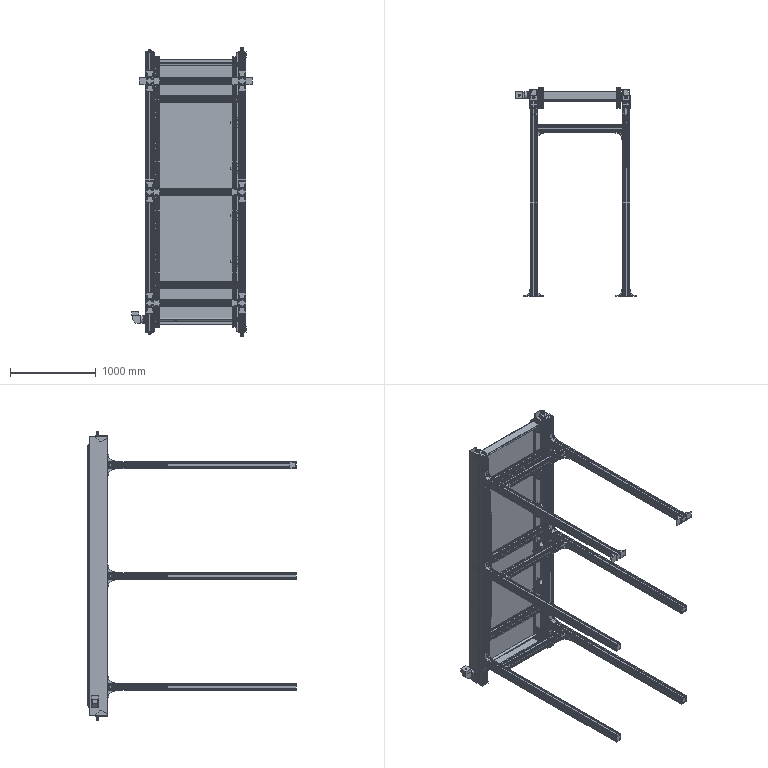Part | NX | features BREP 876 | 1824 solids | 36694 faces | volume 119707773 mm3 | cylinder 18321 | plane 13686 | cone 3061 | torus 870 | sphere 756 | commonest cylinder face diameters 5.96 x5408 18.08 x3746 5.5 x2704 83.184 x2040 11.91 x1352 17.202 x636